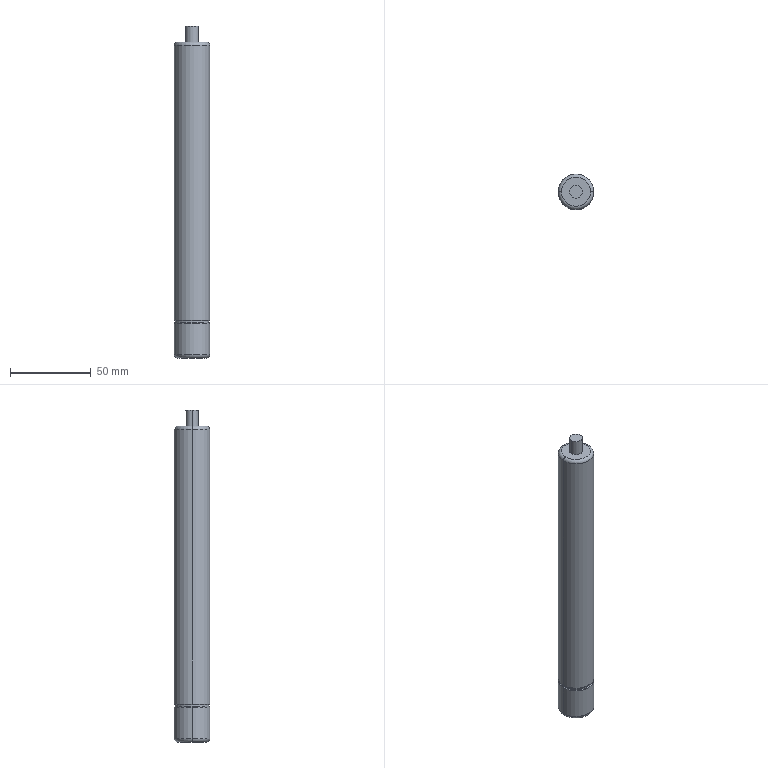Part | SolidWorks | features ICE 3, Fillet 2, Extrusion 1 | 1 solid | 22 faces | box 22 x 22 x 206 mm | volume 60245 mm3 | cylinder 10 | torus 8 | plane 4 | commonest cylinder face diameters 22 x4 8 x2 10 x2 21 x2
STEP:
#1=CARTESIAN_POINT('',(-10.5,0.,22.));
#2=VERTEX_POINT('',#1);
#3=CARTESIAN_POINT('',(10.5,0.,22.));
#4=VERTEX_POINT('',#3);
#5=CARTESIAN_POINT('',(0.,0.,22.));
#6=DIRECTION('',(0.,0.,-1.));
#7=DIRECTION('',(-1.,0.,0.));
#8=AXIS2_PLACEMENT_3D('',#5,#6,#7);
#9=CIRCLE('',#8,10.5);
#10=EDGE_CURVE('',#2,#4,#9,.T.);
#11=ORIENTED_EDGE('',*,*,#10,.T.);
#12=CARTESIAN_POINT('',(11.,0.,21.5));
#13=VERTEX_POINT('',#12);
#14=CARTESIAN_POINT('',(10.5,0.,21.5));
#15=DIRECTION('',(0.,1.,0.));
#16=DIRECTION('',(-1.,0.,0.));
#17=AXIS2_PLACEMENT_3D('',#14,#15,#16);
#18=CIRCLE('',#17,0.5);
#19=EDGE_CURVE('',#4,#13,#18,.T.);
#20=ORIENTED_EDGE('',*,*,#19,.T.);
#21=CARTESIAN_POINT('',(-11.,0.,21.5));
#22=VERTEX_POINT('',#21);
#23=CARTESIAN_POINT('',(0.,0.,21.5));
#24=DIRECTION('',(0.,0.,-1.));
#25=DIRECTION('',(-1.,0.,0.));
#26=AXIS2_PLACEMENT_3D('',#23,#24,#25);
#27=CIRCLE('',#26,11.);
#28=EDGE_CURVE('',#22,#13,#27,.T.);
#29=ORIENTED_EDGE('',*,*,#28,.F.);
#30=CARTESIAN_POINT('',(-10.5,0.,21.5));
#31=DIRECTION('',(0.,-1.,0.));
#32=DIRECTION('',(0.,0.,-1.));
#33=AXIS2_PLACEMENT_3D('',#30,#31,#32);
#34=CIRCLE('',#33,0.5);
#35=EDGE_CURVE('',#2,#22,#34,.T.);
#36=ORIENTED_EDGE('',*,*,#35,.F.);
#37=EDGE_LOOP('',(#11,#20,#29,#36));
#38=FACE_OUTER_BOUND('',#37,.T.);
#39=CARTESIAN_POINT('',(0.,0.,21.5));
#40=DIRECTION('',(0.,0.,-1.));
#41=DIRECTION('',(-1.,0.,0.));
#42=AXIS2_PLACEMENT_3D('',#39,#40,#41);
#43=TOROIDAL_SURFACE('',#42,10.5,0.5);
#44=ADVANCED_FACE('',(#38),#43,.T.);
#45=CARTESIAN_POINT('',(11.,0.,23.5));
#46=VERTEX_POINT('',#45);
#47=CARTESIAN_POINT('',(-11.,0.,23.5));
#48=VERTEX_POINT('',#47);
#49=CARTESIAN_POINT('',(0.,0.,23.5));
#50=DIRECTION('',(0.,0.,1.));
#51=DIRECTION('',(-1.,0.,0.));
#52=AXIS2_PLACEMENT_3D('',#49,#50,#51);
#53=CIRCLE('',#52,11.);
#54=EDGE_CURVE('',#46,#48,#53,.T.);
#55=ORIENTED_EDGE('',*,*,#54,.F.);
#56=CARTESIAN_POINT('',(10.5,0.,23.));
#57=VERTEX_POINT('',#56);
#58=CARTESIAN_POINT('',(10.5,0.,23.5));
#59=DIRECTION('',(0.,1.,0.));
#60=DIRECTION('',(-1.,0.,0.));
#61=AXIS2_PLACEMENT_3D('',#58,#59,#60);
#62=CIRCLE('',#61,0.5);
#63=EDGE_CURVE('',#46,#57,#62,.T.);
#64=ORIENTED_EDGE('',*,*,#63,.T.);
#65=CARTESIAN_POINT('',(-10.5,0.,23.));
#66=VERTEX_POINT('',#65);
#67=CARTESIAN_POINT('',(0.,0.,23.));
#68=DIRECTION('',(0.,0.,-1.));
#69=DIRECTION('',(-1.,0.,0.));
#70=AXIS2_PLACEMENT_3D('',#67,#68,#69);
#71=CIRCLE('',#70,10.5);
#72=EDGE_CURVE('',#66,#57,#71,.T.);
#73=ORIENTED_EDGE('',*,*,#72,.F.);
#74=CARTESIAN_POINT('',(-10.5,0.,23.5));
#75=DIRECTION('',(0.,-1.,0.));
#76=DIRECTION('',(0.,0.,-1.));
#77=AXIS2_PLACEMENT_3D('',#74,#75,#76);
#78=CIRCLE('',#77,0.5);
#79=EDGE_CURVE('',#48,#66,#78,.T.);
#80=ORIENTED_EDGE('',*,*,#79,.F.);
#81=EDGE_LOOP('',(#55,#64,#73,#80));
#82=FACE_OUTER_BOUND('',#81,.T.);
#83=CARTESIAN_POINT('',(0.,0.,23.5));
#84=DIRECTION('',(0.,0.,-1.));
#85=DIRECTION('',(-1.,0.,0.));
#86=AXIS2_PLACEMENT_3D('',#83,#84,#85);
#87=TOROIDAL_SURFACE('',#86,10.5,0.5);
#88=ADVANCED_FACE('',(#82),#87,.T.);
#89=ORIENTED_EDGE('',*,*,#28,.T.);
#90=CARTESIAN_POINT('',(11.,0.,2.));
#91=VERTEX_POINT('',#90);
#92=CARTESIAN_POINT('',(11.,0.,196.));
#93=DIRECTION('',(0.,0.,-1.));
#94=VECTOR('',#93,1000.);
#95=LINE('',#92,#94);
#96=EDGE_CURVE('',#13,#91,#95,.T.);
#97=ORIENTED_EDGE('',*,*,#96,.T.);
#98=CARTESIAN_POINT('',(-11.,0.,2.));
#99=VERTEX_POINT('',#98);
#100=CARTESIAN_POINT('',(0.,0.,2.));
#101=DIRECTION('',(0.,0.,1.));
#102=DIRECTION('',(1.,0.,0.));
#103=AXIS2_PLACEMENT_3D('',#100,#101,#102);
#104=CIRCLE('',#103,11.);
#105=EDGE_CURVE('',#91,#99,#104,.T.);
#106=ORIENTED_EDGE('',*,*,#105,.T.);
#107=CARTESIAN_POINT('',(-11.,0.,196.));
#108=DIRECTION('',(0.,0.,-1.));
#109=VECTOR('',#108,1000.);
#110=LINE('',#107,#109);
#111=EDGE_CURVE('',#22,#99,#110,.T.);
#112=ORIENTED_EDGE('',*,*,#111,.F.);
#113=EDGE_LOOP('',(#89,#97,#106,#112));
#114=FACE_OUTER_BOUND('',#113,.T.);
#115=CARTESIAN_POINT('',(0.,0.,196.));
#116=DIRECTION('',(0.,0.,-1.));
#117=DIRECTION('',(-1.,0.,0.));
#118=AXIS2_PLACEMENT_3D('',#115,#116,#117);
#119=CYLINDRICAL_SURFACE('',#118,11.);
#120=ADVANCED_FACE('',(#114),#119,.T.);
#121=CARTESIAN_POINT('',(-9.,0.,0.));
#122=VERTEX_POINT('',#121);
#123=CARTESIAN_POINT('',(9.,0.,0.));
#124=VERTEX_POINT('',#123);
#125=CARTESIAN_POINT('',(0.,0.,0.));
#126=DIRECTION('',(0.,0.,-1.));
#127=DIRECTION('',(1.,0.,0.));
#128=AXIS2_PLACEMENT_3D('',#125,#126,#127);
#129=CIRCLE('',#128,9.);
#130=EDGE_CURVE('',#122,#124,#129,.T.);
#131=ORIENTED_EDGE('',*,*,#130,.F.);
#132=CARTESIAN_POINT('',(-9.,0.,2.));
#133=DIRECTION('',(0.,1.,0.));
#134=DIRECTION('',(-1.,0.,0.));
#135=AXIS2_PLACEMENT_3D('',#132,#133,#134);
#136=CIRCLE('',#135,2.);
#137=EDGE_CURVE('',#122,#99,#136,.T.);
#138=ORIENTED_EDGE('',*,*,#137,.T.);
#139=ORIENTED_EDGE('',*,*,#105,.F.);
#140=CARTESIAN_POINT('',(9.,0.,2.));
#141=DIRECTION('',(0.,-1.,0.));
#142=DIRECTION('',(0.,0.,-1.));
#143=AXIS2_PLACEMENT_3D('',#140,#141,#142);
#144=CIRCLE('',#143,2.);
#145=EDGE_CURVE('',#124,#91,#144,.T.);
#146=ORIENTED_EDGE('',*,*,#145,.F.);
#147=EDGE_LOOP('',(#131,#138,#139,#146));
#148=FACE_OUTER_BOUND('',#147,.T.);
#149=CARTESIAN_POINT('',(0.,0.,2.));
#150=DIRECTION('',(0.,0.,1.));
#151=DIRECTION('',(1.,0.,0.));
#152=AXIS2_PLACEMENT_3D('',#149,#150,#151);
#153=TOROIDAL_SURFACE('',#152,9.,2.);
#154=ADVANCED_FACE('',(#148),#153,.T.);
#155=CARTESIAN_POINT('',(5.,0.,186.));
#156=VERTEX_POINT('',#155);
#157=CARTESIAN_POINT('',(-5.,0.,186.));
#158=VERTEX_POINT('',#157);
#159=CARTESIAN_POINT('',(0.,0.,186.));
#160=DIRECTION('',(0.,0.,-1.));
#161=DIRECTION('',(-1.,0.,0.));
#162=AXIS2_PLACEMENT_3D('',#159,#160,#161);
#163=CIRCLE('',#162,5.);
#164=EDGE_CURVE('',#156,#158,#163,.T.);
#165=ORIENTED_EDGE('',*,*,#164,.F.);
#166=CARTESIAN_POINT('',(5.,0.,0.));
#167=VERTEX_POINT('',#166);
#168=CARTESIAN_POINT('',(5.,0.,186.));
#169=DIRECTION('',(0.,0.,-1.));
#170=VECTOR('',#169,1000.);
#171=LINE('',#168,#170);
#172=EDGE_CURVE('',#156,#167,#171,.T.);
#173=ORIENTED_EDGE('',*,*,#172,.T.);
#174=CARTESIAN_POINT('',(-5.,0.,0.));
#175=VERTEX_POINT('',#174);
#176=CARTESIAN_POINT('',(0.,0.,0.));
#177=DIRECTION('',(0.,0.,-1.));
#178=DIRECTION('',(-1.,0.,0.));
#179=AXIS2_PLACEMENT_3D('',#176,#177,#178);
#180=CIRCLE('',#179,5.);
#181=EDGE_CURVE('',#167,#175,#180,.T.);
#182=ORIENTED_EDGE('',*,*,#181,.T.);
#183=CARTESIAN_POINT('',(-5.,0.,186.));
#184=DIRECTION('',(0.,0.,-1.));
#185=VECTOR('',#184,1000.);
#186=LINE('',#183,#185);
#187=EDGE_CURVE('',#158,#175,#186,.T.);
#188=ORIENTED_EDGE('',*,*,#187,.F.);
#189=EDGE_LOOP('',(#165,#173,#182,#188));
#190=FACE_OUTER_BOUND('',#189,.T.);
#191=CARTESIAN_POINT('',(0.,0.,186.));
#192=DIRECTION('',(0.,0.,-1.));
#193=DIRECTION('',(-1.,0.,0.));
#194=AXIS2_PLACEMENT_3D('',#191,#192,#193);
#195=CYLINDRICAL_SURFACE('',#194,5.);
#196=ADVANCED_FACE('',(#190),#195,.F.);
#197=ORIENTED_EDGE('',*,*,#72,.T.);
#198=CARTESIAN_POINT('',(10.5,0.,23.));
#199=DIRECTION('',(0.,0.,-1.));
#200=VECTOR('',#199,1000.);
#201=LINE('',#198,#200);
#202=EDGE_CURVE('',#57,#4,#201,.T.);
#203=ORIENTED_EDGE('',*,*,#202,.T.);
#204=ORIENTED_EDGE('',*,*,#10,.F.);
#205=CARTESIAN_POINT('',(-10.5,0.,23.));
#206=DIRECTION('',(0.,0.,-1.));
#207=VECTOR('',#206,1000.);
#208=LINE('',#205,#207);
#209=EDGE_CURVE('',#66,#2,#208,.T.);
#210=ORIENTED_EDGE('',*,*,#209,.F.);
#211=EDGE_LOOP('',(#197,#203,#204,#210));
#212=FACE_OUTER_BOUND('',#211,.T.);
#213=CARTESIAN_POINT('',(0.,0.,23.));
#214=DIRECTION('',(0.,0.,-1.));
#215=DIRECTION('',(-1.,0.,0.));
#216=AXIS2_PLACEMENT_3D('',#213,#214,#215);
#217=CYLINDRICAL_SURFACE('',#216,10.5);
#218=ADVANCED_FACE('',(#212),#217,.T.);
#219=CARTESIAN_POINT('',(-11.,0.,194.));
#220=VERTEX_POINT('',#219);
#221=CARTESIAN_POINT('',(11.,0.,194.));
#222=VERTEX_POINT('',#221);
#223=CARTESIAN_POINT('',(0.,0.,194.));
#224=DIRECTION('',(0.,0.,-1.));
#225=DIRECTION('',(1.,0.,0.));
#226=AXIS2_PLACEMENT_3D('',#223,#224,#225);
#227=CIRCLE('',#226,11.);
#228=EDGE_CURVE('',#220,#222,#227,.T.);
#229=ORIENTED_EDGE('',*,*,#228,.F.);
#230=CARTESIAN_POINT('',(-9.,0.,196.));
#231=VERTEX_POINT('',#230);
#232=CARTESIAN_POINT('',(-9.,0.,194.));
#233=DIRECTION('',(0.,1.,0.));
#234=DIRECTION('',(-1.,0.,0.));
#235=AXIS2_PLACEMENT_3D('',#232,#233,#234);
#236=CIRCLE('',#235,2.);
#237=EDGE_CURVE('',#220,#231,#236,.T.);
#238=ORIENTED_EDGE('',*,*,#237,.T.);
#239=CARTESIAN_POINT('',(9.,0.,196.));
#240=VERTEX_POINT('',#239);
#241=CARTESIAN_POINT('',(0.,0.,196.));
#242=DIRECTION('',(0.,0.,1.));
#243=DIRECTION('',(1.,0.,0.));
#244=AXIS2_PLACEMENT_3D('',#241,#242,#243);
#245=CIRCLE('',#244,9.);
#246=EDGE_CURVE('',#240,#231,#245,.T.);
#247=ORIENTED_EDGE('',*,*,#246,.F.);
#248=CARTESIAN_POINT('',(9.,0.,194.));
#249=DIRECTION('',(0.,-1.,0.));
#250=DIRECTION('',(0.,0.,-1.));
#251=AXIS2_PLACEMENT_3D('',#248,#249,#250);
#252=CIRCLE('',#251,2.);
#253=EDGE_CURVE('',#222,#240,#252,.T.);
#254=ORIENTED_EDGE('',*,*,#253,.F.);
#255=EDGE_LOOP('',(#229,#238,#247,#254));
#256=FACE_OUTER_BOUND('',#255,.T.);
#257=CARTESIAN_POINT('',(0.,0.,194.));
#258=DIRECTION('',(0.,0.,1.));
#259=DIRECTION('',(1.,0.,0.));
#260=AXIS2_PLACEMENT_3D('',#257,#258,#259);
#261=TOROIDAL_SURFACE('',#260,9.,2.);
#262=ADVANCED_FACE('',(#256),#261,.T.);
#263=CARTESIAN_POINT('',(4.,0.,206.));
#264=VERTEX_POINT('',#263);
#265=CARTESIAN_POINT('',(-4.,0.,206.));
#266=VERTEX_POINT('',#265);
#267=CARTESIAN_POINT('',(0.,0.,206.));
#268=DIRECTION('',(0.,0.,1.));
#269=DIRECTION('',(1.,0.,0.));
#270=AXIS2_PLACEMENT_3D('',#267,#268,#269);
#271=CIRCLE('',#270,4.);
#272=EDGE_CURVE('',#264,#266,#271,.T.);
#273=ORIENTED_EDGE('',*,*,#272,.F.);
#274=CARTESIAN_POINT('',(4.,0.,196.));
#275=VERTEX_POINT('',#274);
#276=CARTESIAN_POINT('',(4.,0.,206.));
#277=DIRECTION('',(0.,0.,-1.));
#278=VECTOR('',#277,1000.);
#279=LINE('',#276,#278);
#280=EDGE_CURVE('',#264,#275,#279,.T.);
#281=ORIENTED_EDGE('',*,*,#280,.T.);
#282=CARTESIAN_POINT('',(-4.,0.,196.));
#283=VERTEX_POINT('',#282);
#284=CARTESIAN_POINT('',(0.,0.,196.));
#285=DIRECTION('',(0.,0.,1.));
#286=DIRECTION('',(1.,0.,0.));
#287=AXIS2_PLACEMENT_3D('',#284,#285,#286);
#288=CIRCLE('',#287,4.);
#289=EDGE_CURVE('',#275,#283,#288,.T.);
#290=ORIENTED_EDGE('',*,*,#289,.T.);
#291=CARTESIAN_POINT('',(-4.,0.,206.));
#292=DIRECTION('',(0.,0.,-1.));
#293=VECTOR('',#292,1000.);
#294=LINE('',#291,#293);
#295=EDGE_CURVE('',#266,#283,#294,.T.);
#296=ORIENTED_EDGE('',*,*,#295,.F.);
#297=EDGE_LOOP('',(#273,#281,#290,#296));
#298=FACE_OUTER_BOUND('',#297,.T.);
#299=CARTESIAN_POINT('',(0.,0.,206.));
#300=DIRECTION('',(0.,0.,-1.));
#301=DIRECTION('',(-1.,0.,0.));
#302=AXIS2_PLACEMENT_3D('',#299,#300,#301);
#303=CYLINDRICAL_SURFACE('',#302,4.);
#304=ADVANCED_FACE('',(#298),#303,.T.);
#305=ORIENTED_EDGE('',*,*,#228,.T.);
#306=CARTESIAN_POINT('',(11.,0.,196.));
#307=DIRECTION('',(0.,0.,-1.));
#308=VECTOR('',#307,1000.);
#309=LINE('',#306,#308);
#310=EDGE_CURVE('',#222,#46,#309,.T.);
#311=ORIENTED_EDGE('',*,*,#310,.T.);
#312=ORIENTED_EDGE('',*,*,#54,.T.);
#313=CARTESIAN_POINT('',(-11.,0.,196.));
#314=DIRECTION('',(0.,0.,-1.));
#315=VECTOR('',#314,1000.);
#316=LINE('',#313,#315);
#317=EDGE_CURVE('',#220,#48,#316,.T.);
#318=ORIENTED_EDGE('',*,*,#317,.F.);
#319=EDGE_LOOP('',(#305,#311,#312,#318));
#320=FACE_OUTER_BOUND('',#319,.T.);
#321=CARTESIAN_POINT('',(0.,0.,196.));
#322=DIRECTION('',(0.,0.,-1.));
#323=DIRECTION('',(-1.,0.,0.));
#324=AXIS2_PLACEMENT_3D('',#321,#322,#323);
#325=CYLINDRICAL_SURFACE('',#324,11.);
#326=ADVANCED_FACE('',(#320),#325,.T.);
#327=ORIENTED_EDGE('',*,*,#310,.F.);
#328=CARTESIAN_POINT('',(0.,0.,194.));
#329=DIRECTION('',(0.,0.,-1.));
#330=DIRECTION('',(1.,0.,0.));
#331=AXIS2_PLACEMENT_3D('',#328,#329,#330);
#332=CIRCLE('',#331,11.);
#333=EDGE_CURVE('',#222,#220,#332,.T.);
#334=ORIENTED_EDGE('',*,*,#333,.T.);
#335=ORIENTED_EDGE('',*,*,#317,.T.);
#336=CARTESIAN_POINT('',(0.,0.,23.5));
#337=DIRECTION('',(0.,0.,1.));
#338=DIRECTION('',(-1.,0.,0.));
#339=AXIS2_PLACEMENT_3D('',#336,#337,#338);
#340=CIRCLE('',#339,11.);
#341=EDGE_CURVE('',#48,#46,#340,.T.);
#342=ORIENTED_EDGE('',*,*,#341,.T.);
#343=EDGE_LOOP('',(#327,#334,#335,#342));
#344=FACE_OUTER_BOUND('',#343,.T.);
#345=CARTESIAN_POINT('',(0.,0.,196.));
#346=DIRECTION('',(0.,0.,-1.));
#347=DIRECTION('',(-1.,0.,0.));
#348=AXIS2_PLACEMENT_3D('',#345,#346,#347);
#349=CYLINDRICAL_SURFACE('',#348,11.);
#350=ADVANCED_FACE('',(#344),#349,.T.);
#351=ORIENTED_EDGE('',*,*,#246,.T.);
#352=CARTESIAN_POINT('',(0.,0.,196.));
#353=DIRECTION('',(0.,0.,1.));
#354=DIRECTION('',(1.,0.,0.));
#355=AXIS2_PLACEMENT_3D('',#352,#353,#354);
#356=CIRCLE('',#355,9.);
#357=EDGE_CURVE('',#231,#240,#356,.T.);
#358=ORIENTED_EDGE('',*,*,#357,.T.);
#359=EDGE_LOOP('',(#351,#358));
#360=FACE_OUTER_BOUND('',#359,.T.);
#361=CARTESIAN_POINT('',(0.,0.,196.));
#362=DIRECTION('',(0.,0.,1.));
#363=DIRECTION('',(1.,0.,0.));
#364=AXIS2_PLACEMENT_3D('',#361,#362,#363);
#365=CIRCLE('',#364,4.);
#366=EDGE_CURVE('',#283,#275,#365,.T.);
#367=ORIENTED_EDGE('',*,*,#366,.F.);
#368=ORIENTED_EDGE('',*,*,#289,.F.);
#369=EDGE_LOOP('',(#367,#368));
#370=FACE_BOUND('',#369,.T.);
#371=CARTESIAN_POINT('',(0.,0.,196.));
#372=DIRECTION('',(0.,0.,1.));
#373=DIRECTION('',(1.,0.,0.));
#374=AXIS2_PLACEMENT_3D('',#371,#372,#373);
#375=PLANE('',#374);
#376=ADVANCED_FACE('',(#360,#370),#375,.T.);
#377=ORIENTED_EDGE('',*,*,#280,.F.);
#378=CARTESIAN_POINT('',(0.,0.,206.));
#379=DIRECTION('',(0.,0.,1.));
#380=DIRECTION('',(1.,0.,0.));
#381=AXIS2_PLACEMENT_3D('',#378,#379,#380);
#382=CIRCLE('',#381,4.);
#383=EDGE_CURVE('',#266,#264,#382,.T.);
#384=ORIENTED_EDGE('',*,*,#383,.F.);
#385=ORIENTED_EDGE('',*,*,#295,.T.);
#386=ORIENTED_EDGE('',*,*,#366,.T.);
#387=EDGE_LOOP('',(#377,#384,#385,#386));
#388=FACE_OUTER_BOUND('',#387,.T.);
#389=CARTESIAN_POINT('',(0.,0.,206.));
#390=DIRECTION('',(0.,0.,-1.));
#391=DIRECTION('',(-1.,0.,0.));
#392=AXIS2_PLACEMENT_3D('',#389,#390,#391);
#393=CYLINDRICAL_SURFACE('',#392,4.);
#394=ADVANCED_FACE('',(#388),#393,.T.);
#395=ORIENTED_EDGE('',*,*,#383,.T.);
#396=ORIENTED_EDGE('',*,*,#272,.T.);
#397=EDGE_LOOP('',(#395,#396));
#398=FACE_OUTER_BOUND('',#397,.T.);
#399=CARTESIAN_POINT('',(0.,0.,206.));
#400=DIRECTION('',(0.,0.,1.));
#401=DIRECTION('',(1.,0.,0.));
#402=AXIS2_PLACEMENT_3D('',#399,#400,#401);
#403=PLANE('',#402);
#404=ADVANCED_FACE('',(#398),#403,.T.);
#405=ORIENTED_EDGE('',*,*,#237,.F.);
#406=ORIENTED_EDGE('',*,*,#333,.F.);
#407=ORIENTED_EDGE('',*,*,#253,.T.);
#408=ORIENTED_EDGE('',*,*,#357,.F.);
#409=EDGE_LOOP('',(#405,#406,#407,#408));
#410=FACE_OUTER_BOUND('',#409,.T.);
#411=CARTESIAN_POINT('',(0.,0.,194.));
#412=DIRECTION('',(0.,0.,1.));
#413=DIRECTION('',(1.,0.,0.));
#414=AXIS2_PLACEMENT_3D('',#411,#412,#413);
#415=TOROIDAL_SURFACE('',#414,9.,2.);
#416=ADVANCED_FACE('',(#410),#415,.T.);
#417=ORIENTED_EDGE('',*,*,#202,.F.);
#418=CARTESIAN_POINT('',(0.,0.,23.));
#419=DIRECTION('',(0.,0.,-1.));
#420=DIRECTION('',(-1.,0.,0.));
#421=AXIS2_PLACEMENT_3D('',#418,#419,#420);
#422=CIRCLE('',#421,10.5);
#423=EDGE_CURVE('',#57,#66,#422,.T.);
#424=ORIENTED_EDGE('',*,*,#423,.T.);
#425=ORIENTED_EDGE('',*,*,#209,.T.);
#426=CARTESIAN_POINT('',(0.,0.,22.));
#427=DIRECTION('',(0.,0.,-1.));
#428=DIRECTION('',(-1.,0.,0.));
#429=AXIS2_PLACEMENT_3D('',#426,#427,#428);
#430=CIRCLE('',#429,10.5);
#431=EDGE_CURVE('',#4,#2,#430,.T.);
#432=ORIENTED_EDGE('',*,*,#431,.F.);
#433=EDGE_LOOP('',(#417,#424,#425,#432));
#434=FACE_OUTER_BOUND('',#433,.T.);
#435=CARTESIAN_POINT('',(0.,0.,23.));
#436=DIRECTION('',(0.,0.,-1.));
#437=DIRECTION('',(-1.,0.,0.));
#438=AXIS2_PLACEMENT_3D('',#435,#436,#437);
#439=CYLINDRICAL_SURFACE('',#438,10.5);
#440=ADVANCED_FACE('',(#434),#439,.T.);
#441=CARTESIAN_POINT('',(0.,0.,186.));
#442=DIRECTION('',(0.,0.,-1.));
#443=DIRECTION('',(-1.,0.,0.));
#444=AXIS2_PLACEMENT_3D('',#441,#442,#443);
#445=CIRCLE('',#444,5.);
#446=EDGE_CURVE('',#158,#156,#445,.T.);
#447=ORIENTED_EDGE('',*,*,#446,.T.);
#448=ORIENTED_EDGE('',*,*,#164,.T.);
#449=EDGE_LOOP('',(#447,#448));
#450=FACE_OUTER_BOUND('',#449,.T.);
#451=CARTESIAN_POINT('',(0.,0.,186.));
#452=DIRECTION('',(0.,0.,-1.));
#453=DIRECTION('',(-1.,0.,0.));
#454=AXIS2_PLACEMENT_3D('',#451,#452,#453);
#455=PLANE('',#454);
#456=ADVANCED_FACE('',(#450),#455,.T.);
#457=ORIENTED_EDGE('',*,*,#172,.F.);
#458=ORIENTED_EDGE('',*,*,#446,.F.);
#459=ORIENTED_EDGE('',*,*,#187,.T.);
#460=CARTESIAN_POINT('',(0.,0.,0.));
#461=DIRECTION('',(0.,0.,-1.));
#462=DIRECTION('',(-1.,0.,0.));
#463=AXIS2_PLACEMENT_3D('',#460,#461,#462);
#464=CIRCLE('',#463,5.);
#465=EDGE_CURVE('',#175,#167,#464,.T.);
#466=ORIENTED_EDGE('',*,*,#465,.T.);
#467=EDGE_LOOP('',(#457,#458,#459,#466));
#468=FACE_OUTER_BOUND('',#467,.T.);
#469=CARTESIAN_POINT('',(0.,0.,186.));
#470=DIRECTION('',(0.,0.,-1.));
#471=DIRECTION('',(-1.,0.,0.));
#472=AXIS2_PLACEMENT_3D('',#469,#470,#471);
#473=CYLINDRICAL_SURFACE('',#472,5.);
#474=ADVANCED_FACE('',(#468),#473,.F.);
#475=CARTESIAN_POINT('',(0.,0.,0.));
#476=DIRECTION('',(0.,0.,-1.));
#477=DIRECTION('',(1.,0.,0.));
#478=AXIS2_PLACEMENT_3D('',#475,#476,#477);
#479=CIRCLE('',#478,9.);
#480=EDGE_CURVE('',#124,#122,#479,.T.);
#481=ORIENTED_EDGE('',*,*,#480,.T.);
#482=ORIENTED_EDGE('',*,*,#130,.T.);
#483=EDGE_LOOP('',(#481,#482));
#484=FACE_OUTER_BOUND('',#483,.T.);
#485=ORIENTED_EDGE('',*,*,#465,.F.);
#486=ORIENTED_EDGE('',*,*,#181,.F.);
#487=EDGE_LOOP('',(#485,#486));
#488=FACE_BOUND('',#487,.T.);
#489=CARTESIAN_POINT('',(0.,0.,0.));
#490=DIRECTION('',(0.,0.,1.));
#491=DIRECTION('',(1.,0.,0.));
#492=AXIS2_PLACEMENT_3D('',#489,#490,#491);
#493=PLANE('',#492);
#494=ADVANCED_FACE('',(#484,#488),#493,.F.);
#495=ORIENTED_EDGE('',*,*,#137,.F.);
#496=ORIENTED_EDGE('',*,*,#480,.F.);
#497=ORIENTED_EDGE('',*,*,#145,.T.);
#498=CARTESIAN_POINT('',(0.,0.,2.));
#499=DIRECTION('',(0.,0.,1.));
#500=DIRECTION('',(1.,0.,0.));
#501=AXIS2_PLACEMENT_3D('',#498,#499,#500);
#502=CIRCLE('',#501,11.);
#503=EDGE_CURVE('',#99,#91,#502,.T.);
#504=ORIENTED_EDGE('',*,*,#503,.F.);
#505=EDGE_LOOP('',(#495,#496,#497,#504));
#506=FACE_OUTER_BOUND('',#505,.T.);
#507=CARTESIAN_POINT('',(0.,0.,2.));
#508=DIRECTION('',(0.,0.,1.));
#509=DIRECTION('',(1.,0.,0.));
#510=AXIS2_PLACEMENT_3D('',#507,#508,#509);
#511=TOROIDAL_SURFACE('',#510,9.,2.);
#512=ADVANCED_FACE('',(#506),#511,.T.);
#513=ORIENTED_EDGE('',*,*,#96,.F.);
#514=CARTESIAN_POINT('',(0.,0.,21.5));
#515=DIRECTION('',(0.,0.,-1.));
#516=DIRECTION('',(-1.,0.,0.));
#517=AXIS2_PLACEMENT_3D('',#514,#515,#516);
#518=CIRCLE('',#517,11.);
#519=EDGE_CURVE('',#13,#22,#518,.T.);
#520=ORIENTED_EDGE('',*,*,#519,.T.);
#521=ORIENTED_EDGE('',*,*,#111,.T.);
#522=ORIENTED_EDGE('',*,*,#503,.T.);
#523=EDGE_LOOP('',(#513,#520,#521,#522));
#524=FACE_OUTER_BOUND('',#523,.T.);
#525=CARTESIAN_POINT('',(0.,0.,196.));
#526=DIRECTION('',(0.,0.,-1.));
#527=DIRECTION('',(-1.,0.,0.));
#528=AXIS2_PLACEMENT_3D('',#525,#526,#527);
#529=CYLINDRICAL_SURFACE('',#528,11.);
#530=ADVANCED_FACE('',(#524),#529,.T.);
#531=ORIENTED_EDGE('',*,*,#63,.F.);
#532=ORIENTED_EDGE('',*,*,#341,.F.);
#533=ORIENTED_EDGE('',*,*,#79,.T.);
#534=ORIENTED_EDGE('',*,*,#423,.F.);
#535=EDGE_LOOP('',(#531,#532,#533,#534));
#536=FACE_OUTER_BOUND('',#535,.T.);
#537=CARTESIAN_POINT('',(0.,0.,23.5));
#538=DIRECTION('',(0.,0.,-1.));
#539=DIRECTION('',(-1.,0.,0.));
#540=AXIS2_PLACEMENT_3D('',#537,#538,#539);
#541=TOROIDAL_SURFACE('',#540,10.5,0.5);
#542=ADVANCED_FACE('',(#536),#541,.T.);
#543=ORIENTED_EDGE('',*,*,#19,.F.);
#544=ORIENTED_EDGE('',*,*,#431,.T.);
#545=ORIENTED_EDGE('',*,*,#35,.T.);
#546=ORIENTED_EDGE('',*,*,#519,.F.);
#547=EDGE_LOOP('',(#543,#544,#545,#546));
#548=FACE_OUTER_BOUND('',#547,.T.);
#549=CARTESIAN_POINT('',(0.,0.,21.5));
#550=DIRECTION('',(0.,0.,-1.));
#551=DIRECTION('',(-1.,0.,0.));
#552=AXIS2_PLACEMENT_3D('',#549,#550,#551);
#553=TOROIDAL_SURFACE('',#552,10.5,0.5);
#554=ADVANCED_FACE('',(#548),#553,.T.);
#555=CLOSED_SHELL('',(#44,#88,#120,#154,#196,#218,#262,#304,#326,#350,#376,#394,#404,#416,#440,#456,#474,#494,#512,#530,#542,#554));
#556=MANIFOLD_SOLID_BREP('',#555);
#557=CARTESIAN_POINT('',(0.,0.,0.));
#558=DIRECTION('',(0.,0.,1.));
#559=DIRECTION('',(1.,0.,0.));
#560=AXIS2_PLACEMENT_3D('',#557,#558,#559);
#561=(LENGTH_UNIT()NAMED_UNIT(*)SI_UNIT(.MILLI.,.METRE.));
#562=UNCERTAINTY_MEASURE_WITH_UNIT(LENGTH_MEASURE(0.00001),#561,'','');
#563=(NAMED_UNIT(*)PLANE_ANGLE_UNIT()SI_UNIT($,.RADIAN.));
#564=(NAMED_UNIT(*)SI_UNIT($,.STERADIAN.)SOLID_ANGLE_UNIT());
#565=(GEOMETRIC_REPRESENTATION_CONTEXT(3)GLOBAL_UNCERTAINTY_ASSIGNED_CONTEXT((#562))GLOBAL_UNIT_ASSIGNED_CONTEXT((#561,#563,#564))REPRESENTATION_CONTEXT('',''));
#566=ADVANCED_BREP_SHAPE_REPRESENTATION('',(#556,#560),#565);